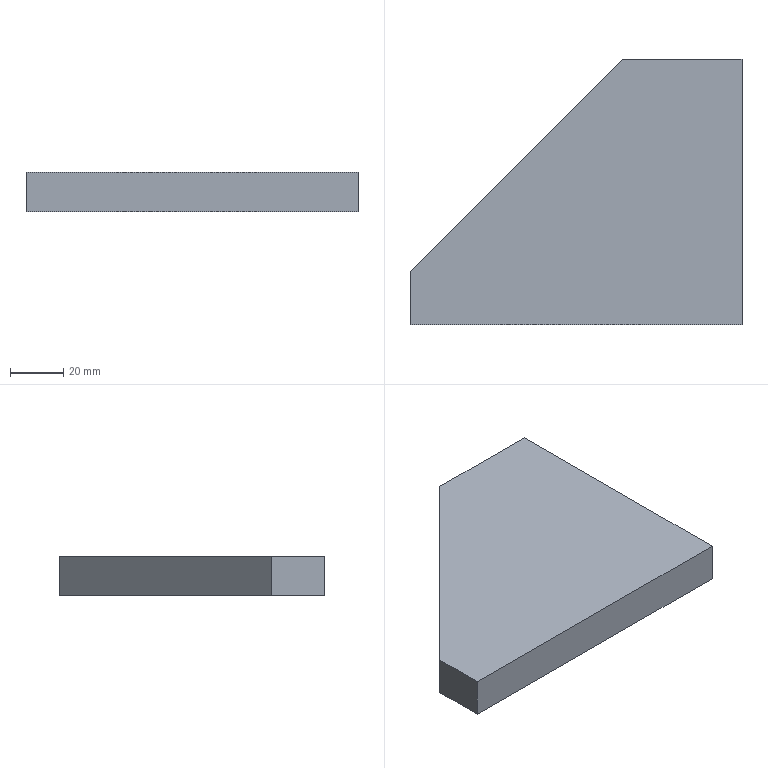Part | SolidWorks | features Chamfer 1, Extrusion 1 | 1 solid | 7 faces | box 125 x 100 x 15 mm | volume 139500 mm3 | plane 7
STEP:
#1=CARTESIAN_POINT('',(62.5,-50.,0.));
#2=VERTEX_POINT('',#1);
#3=CARTESIAN_POINT('',(62.5,50.,0.));
#4=VERTEX_POINT('',#3);
#5=CARTESIAN_POINT('',(62.5,-50.,0.));
#6=DIRECTION('',(0.,1.,0.));
#7=VECTOR('',#6,1000.);
#8=LINE('',#5,#7);
#9=EDGE_CURVE('',#2,#4,#8,.T.);
#10=ORIENTED_EDGE('',*,*,#9,.T.);
#11=CARTESIAN_POINT('',(62.5,50.,15.));
#12=VERTEX_POINT('',#11);
#13=CARTESIAN_POINT('',(62.5,50.,15.));
#14=DIRECTION('',(0.,0.,-1.));
#15=VECTOR('',#14,1000.);
#16=LINE('',#13,#15);
#17=EDGE_CURVE('',#12,#4,#16,.T.);
#18=ORIENTED_EDGE('',*,*,#17,.F.);
#19=CARTESIAN_POINT('',(62.5,-50.,15.));
#20=VERTEX_POINT('',#19);
#21=CARTESIAN_POINT('',(62.5,-50.,15.));
#22=DIRECTION('',(0.,1.,0.));
#23=VECTOR('',#22,1000.);
#24=LINE('',#21,#23);
#25=EDGE_CURVE('',#20,#12,#24,.T.);
#26=ORIENTED_EDGE('',*,*,#25,.F.);
#27=CARTESIAN_POINT('',(62.5,-50.,15.));
#28=DIRECTION('',(0.,0.,-1.));
#29=VECTOR('',#28,1000.);
#30=LINE('',#27,#29);
#31=EDGE_CURVE('',#20,#2,#30,.T.);
#32=ORIENTED_EDGE('',*,*,#31,.T.);
#33=EDGE_LOOP('',(#10,#18,#26,#32));
#34=FACE_OUTER_BOUND('',#33,.T.);
#35=CARTESIAN_POINT('',(62.5,-50.,15.));
#36=DIRECTION('',(-1.,0.,0.));
#37=DIRECTION('',(0.,0.,1.));
#38=AXIS2_PLACEMENT_3D('',#35,#36,#37);
#39=PLANE('',#38);
#40=ADVANCED_FACE('',(#34),#39,.F.);
#41=CARTESIAN_POINT('',(17.5,50.,0.));
#42=VERTEX_POINT('',#41);
#43=CARTESIAN_POINT('',(-62.5,50.,0.));
#44=DIRECTION('',(-1.,0.,0.));
#45=VECTOR('',#44,1000.);
#46=LINE('',#43,#45);
#47=EDGE_CURVE('',#4,#42,#46,.T.);
#48=ORIENTED_EDGE('',*,*,#47,.T.);
#49=CARTESIAN_POINT('',(17.5,50.,15.));
#50=VERTEX_POINT('',#49);
#51=CARTESIAN_POINT('',(17.5,50.,15.));
#52=DIRECTION('',(0.,0.,1.));
#53=VECTOR('',#52,1000.);
#54=LINE('',#51,#53);
#55=EDGE_CURVE('',#42,#50,#54,.T.);
#56=ORIENTED_EDGE('',*,*,#55,.T.);
#57=CARTESIAN_POINT('',(-62.5,50.,15.));
#58=DIRECTION('',(-1.,0.,0.));
#59=VECTOR('',#58,1000.);
#60=LINE('',#57,#59);
#61=EDGE_CURVE('',#12,#50,#60,.T.);
#62=ORIENTED_EDGE('',*,*,#61,.F.);
#63=ORIENTED_EDGE('',*,*,#17,.T.);
#64=EDGE_LOOP('',(#48,#56,#62,#63));
#65=FACE_OUTER_BOUND('',#64,.T.);
#66=CARTESIAN_POINT('',(-62.5,50.,15.));
#67=DIRECTION('',(0.,-1.,0.));
#68=DIRECTION('',(0.,0.,-1.));
#69=AXIS2_PLACEMENT_3D('',#66,#67,#68);
#70=PLANE('',#69);
#71=ADVANCED_FACE('',(#65),#70,.F.);
#72=CARTESIAN_POINT('',(-62.5,-30.,15.));
#73=VERTEX_POINT('',#72);
#74=CARTESIAN_POINT('',(-62.5,-50.,15.));
#75=VERTEX_POINT('',#74);
#76=CARTESIAN_POINT('',(-62.5,-50.,15.));
#77=DIRECTION('',(0.,-1.,0.));
#78=VECTOR('',#77,1000.);
#79=LINE('',#76,#78);
#80=EDGE_CURVE('',#73,#75,#79,.T.);
#81=ORIENTED_EDGE('',*,*,#80,.F.);
#82=CARTESIAN_POINT('',(-62.5,-30.,0.));
#83=VERTEX_POINT('',#82);
#84=CARTESIAN_POINT('',(-62.5,-30.,15.));
#85=DIRECTION('',(0.,0.,-1.));
#86=VECTOR('',#85,1000.);
#87=LINE('',#84,#86);
#88=EDGE_CURVE('',#73,#83,#87,.T.);
#89=ORIENTED_EDGE('',*,*,#88,.T.);
#90=CARTESIAN_POINT('',(-62.5,-50.,0.));
#91=VERTEX_POINT('',#90);
#92=CARTESIAN_POINT('',(-62.5,-50.,0.));
#93=DIRECTION('',(0.,-1.,0.));
#94=VECTOR('',#93,1000.);
#95=LINE('',#92,#94);
#96=EDGE_CURVE('',#83,#91,#95,.T.);
#97=ORIENTED_EDGE('',*,*,#96,.T.);
#98=CARTESIAN_POINT('',(-62.5,-50.,15.));
#99=DIRECTION('',(0.,0.,-1.));
#100=VECTOR('',#99,1000.);
#101=LINE('',#98,#100);
#102=EDGE_CURVE('',#75,#91,#101,.T.);
#103=ORIENTED_EDGE('',*,*,#102,.F.);
#104=EDGE_LOOP('',(#81,#89,#97,#103));
#105=FACE_OUTER_BOUND('',#104,.T.);
#106=CARTESIAN_POINT('',(-62.5,-50.,15.));
#107=DIRECTION('',(1.,0.,0.));
#108=DIRECTION('',(0.,0.,-1.));
#109=AXIS2_PLACEMENT_3D('',#106,#107,#108);
#110=PLANE('',#109);
#111=ADVANCED_FACE('',(#105),#110,.F.);
#112=CARTESIAN_POINT('',(-62.5,-50.,0.));
#113=DIRECTION('',(1.,0.,0.));
#114=VECTOR('',#113,1000.);
#115=LINE('',#112,#114);
#116=EDGE_CURVE('',#91,#2,#115,.T.);
#117=ORIENTED_EDGE('',*,*,#116,.T.);
#118=ORIENTED_EDGE('',*,*,#31,.F.);
#119=CARTESIAN_POINT('',(-62.5,-50.,15.));
#120=DIRECTION('',(1.,0.,0.));
#121=VECTOR('',#120,1000.);
#122=LINE('',#119,#121);
#123=EDGE_CURVE('',#75,#20,#122,.T.);
#124=ORIENTED_EDGE('',*,*,#123,.F.);
#125=ORIENTED_EDGE('',*,*,#102,.T.);
#126=EDGE_LOOP('',(#117,#118,#124,#125));
#127=FACE_OUTER_BOUND('',#126,.T.);
#128=CARTESIAN_POINT('',(-62.5,-50.,15.));
#129=DIRECTION('',(0.,1.,0.));
#130=DIRECTION('',(0.,0.,1.));
#131=AXIS2_PLACEMENT_3D('',#128,#129,#130);
#132=PLANE('',#131);
#133=ADVANCED_FACE('',(#127),#132,.F.);
#134=ORIENTED_EDGE('',*,*,#61,.T.);
#135=CARTESIAN_POINT('',(-62.5,-30.,15.));
#136=DIRECTION('',(-0.7071,-0.7071,0.));
#137=VECTOR('',#136,1000.);
#138=LINE('',#135,#137);
#139=EDGE_CURVE('',#50,#73,#138,.T.);
#140=ORIENTED_EDGE('',*,*,#139,.T.);
#141=ORIENTED_EDGE('',*,*,#80,.T.);
#142=ORIENTED_EDGE('',*,*,#123,.T.);
#143=ORIENTED_EDGE('',*,*,#25,.T.);
#144=EDGE_LOOP('',(#134,#140,#141,#142,#143));
#145=FACE_OUTER_BOUND('',#144,.T.);
#146=CARTESIAN_POINT('',(0.,0.,15.));
#147=DIRECTION('',(0.,0.,-1.));
#148=DIRECTION('',(-1.,0.,0.));
#149=AXIS2_PLACEMENT_3D('',#146,#147,#148);
#150=PLANE('',#149);
#151=ADVANCED_FACE('',(#145),#150,.F.);
#152=ORIENTED_EDGE('',*,*,#96,.F.);
#153=CARTESIAN_POINT('',(-16.25,16.25,0.));
#154=DIRECTION('',(0.7071,0.7071,0.));
#155=VECTOR('',#154,1000.);
#156=LINE('',#153,#155);
#157=EDGE_CURVE('',#83,#42,#156,.T.);
#158=ORIENTED_EDGE('',*,*,#157,.T.);
#159=ORIENTED_EDGE('',*,*,#47,.F.);
#160=ORIENTED_EDGE('',*,*,#9,.F.);
#161=ORIENTED_EDGE('',*,*,#116,.F.);
#162=EDGE_LOOP('',(#152,#158,#159,#160,#161));
#163=FACE_OUTER_BOUND('',#162,.T.);
#164=CARTESIAN_POINT('',(0.,0.,0.));
#165=DIRECTION('',(0.,0.,-1.));
#166=DIRECTION('',(-1.,0.,0.));
#167=AXIS2_PLACEMENT_3D('',#164,#165,#166);
#168=PLANE('',#167);
#169=ADVANCED_FACE('',(#163),#168,.T.);
#170=ORIENTED_EDGE('',*,*,#139,.F.);
#171=ORIENTED_EDGE('',*,*,#55,.F.);
#172=ORIENTED_EDGE('',*,*,#157,.F.);
#173=ORIENTED_EDGE('',*,*,#88,.F.);
#174=EDGE_LOOP('',(#170,#171,#172,#173));
#175=FACE_OUTER_BOUND('',#174,.T.);
#176=CARTESIAN_POINT('',(-62.5,-30.,15.));
#177=DIRECTION('',(0.7071,-0.7071,0.));
#178=DIRECTION('',(0.,0.,-1.));
#179=AXIS2_PLACEMENT_3D('',#176,#177,#178);
#180=PLANE('',#179);
#181=ADVANCED_FACE('',(#175),#180,.F.);
#182=CLOSED_SHELL('',(#40,#71,#111,#133,#151,#169,#181));
#183=MANIFOLD_SOLID_BREP('',#182);
#184=CARTESIAN_POINT('',(0.,0.,0.));
#185=DIRECTION('',(0.,0.,1.));
#186=DIRECTION('',(1.,0.,0.));
#187=AXIS2_PLACEMENT_3D('',#184,#185,#186);
#188=(LENGTH_UNIT()NAMED_UNIT(*)SI_UNIT(.MILLI.,.METRE.));
#189=UNCERTAINTY_MEASURE_WITH_UNIT(LENGTH_MEASURE(0.00001),#188,'','');
#190=(NAMED_UNIT(*)PLANE_ANGLE_UNIT()SI_UNIT($,.RADIAN.));
#191=(NAMED_UNIT(*)SI_UNIT($,.STERADIAN.)SOLID_ANGLE_UNIT());
#192=(GEOMETRIC_REPRESENTATION_CONTEXT(3)GLOBAL_UNCERTAINTY_ASSIGNED_CONTEXT((#189))GLOBAL_UNIT_ASSIGNED_CONTEXT((#188,#190,#191))REPRESENTATION_CONTEXT('',''));
#193=ADVANCED_BREP_SHAPE_REPRESENTATION('',(#183,#187),#192);